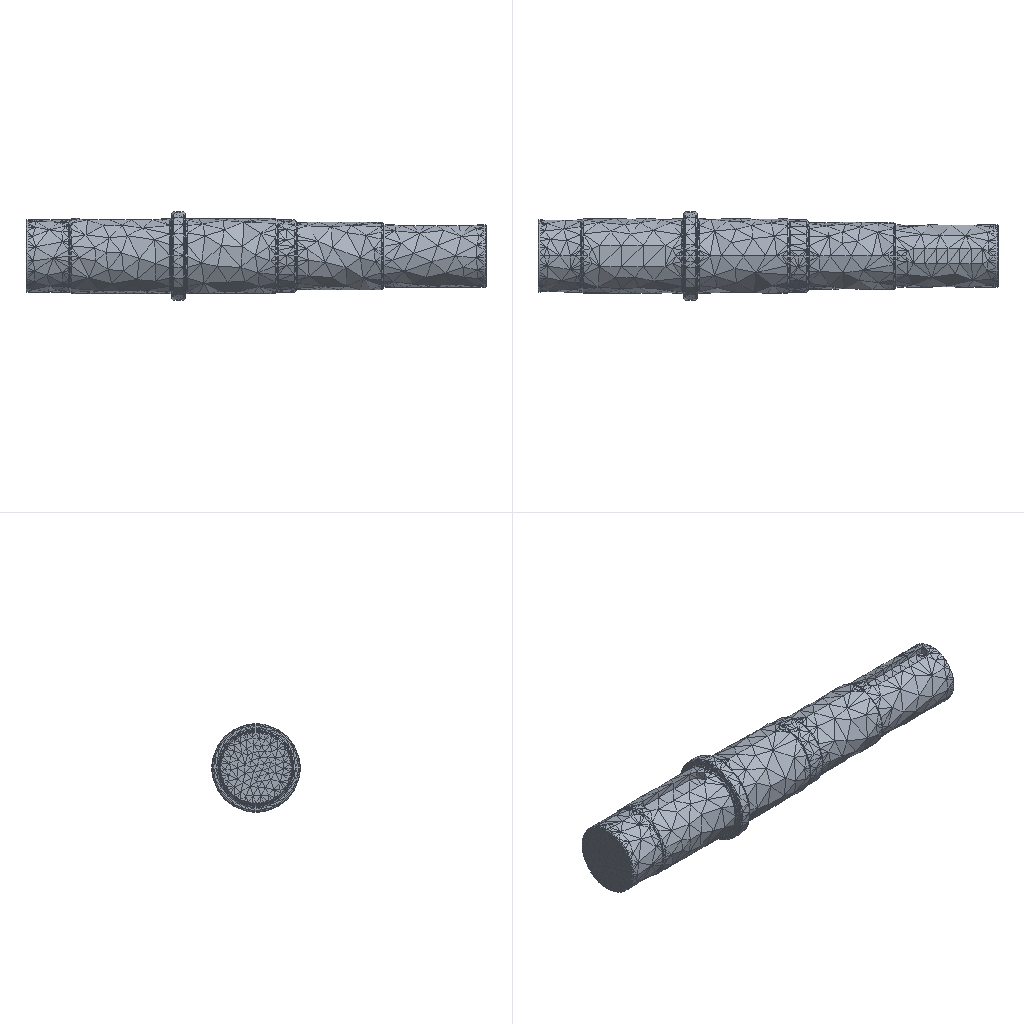Simulation study | ansys workbench
Ansys APDL input file, long lists of numbers shortened:
/batch
/config,noeldb,1     ! force off writing results to database
*get,_wallstrt,active,,time,wall
! ANSYS input file written by Workbench version 2022 R1
! File used for geometry attach: F:\ansys（分析文件汇总)\轴有限元分析222\三轴.STEP
/title,1--____ (B5)
! ****** Begin Custom Load Command Snippet ******
/COM, ACT Extensions:
/COM,     LSDYNA, 2021.1
/COM,
! ****** End   Custom Load Command Snippet ******
*DIM,_wb_ProjectScratch_dir,string,248
_wb_ProjectScratch_dir(1) = 'F:\ansys（分析文件汇总)\轴有限元分析222\_ProjectScratch\Scr97E6\'
*DIM,_wb_SolverFiles_dir,string,248
_wb_SolverFiles_dir(1) = 'F:\ansys（分析文件汇总)\轴有限元分析222\1_files\dp0\SYS\MECH\'
*DIM,_wb_userfiles_dir,string,248
_wb_userfiles_dir(1) = 'F:\ansys（分析文件汇总)\轴有限元分析222\1_files\user_files\'
/com,--- Data in consistent NMM units. See Solving Units in the help system for more information.
/units,MPA
/nopr
/wb,file,start              !  signify a WB generated input file
/prep7
! Turn off shape checking because checks already performed inside WB mesher.
! See help system for more information.
SHPP,OFF,,NOWARN
/nolist
etcon,set             ! allow ANSYS to choose best KEYOP's for 180x elements, resets any applicable keyopt to MAPDL defaults
/com,*********** Nodes for the whole assembly ***********
nblock,3,,12992
(1i9,3e20.9e3)
        1     1.495000000E+02     6.024925164E-25    -3.900000000E+01
! (11810 more lines like these left out)
-1
/com,*********** Nodes for all Remote Points ***********
nblock,3
(1i9,3e20.9e3)
    11812     2.186806849E+02    -4.529709940E-14    -2.585144555E-16
-1
/wb,elem,start            !  set before creation of elements
/com,*********** Elements for Body 1 "__-FreeParts|0:35179" ***********
et,1,187
eblock,19,solid,,6720
(19i9)
        1        1        1        1        0        0        0        0       10        0        1      349     1869      691     1621     4224     6255     4217     4221
! (13439 more lines like these left out)
-1
/wb,elem,end               !  done creating elements
/com,*********** Send User Defined Coordinate System(s) ***********
csys,0
toffst,273.15,  ! Temperature offset from absolute zero
/com,*********** Set Reference Temperature ***********
tref,22.
/wb,mat,start              !  starting to send materials
/com,*********** Send Materials ***********
Temperature = 'TEMP' ! Temperature
MP,DENS,1,7.85e-09,	! tonne mm^-3
MP,ALPX,1,1.2e-05,	! C^-1
MP,C,1,434000000,	! mm^2 s^-2 C^-1
MP,KXX,1,60.5,	! tonne mm s^-3 C^-1
MP,RSVX,1,0.00017,	! ohm mm
MP,EX,1,200000,	! tonne s^-2 mm^-1
MP,NUXY,1,0.3,
MP,MURX,1,10000,
/wb,mat,end                !  done sending materials
!************************* Model Summary ********************
!__-FreeParts|0:35179,	结构钢,	matid,	1
!************************* End Model Summary ********************
! get the diagonal of the bounding box. Needed later for other things
*get,_xmin,node,,mnloc,x
*get,_ymin,node,,mnloc,y
*get,_zmin,node,,mnloc,z
*get,_xmax,node,,mxloc,x
*get,_ymax,node,,mxloc,y
*get,_zmax,node,,mxloc,z
_ASMDIAG=(_xmax-_xmin)*(_xmax-_xmin)+(_ymax-_ymin)*(_ymax-_ymin)+(_zmax-_zmin)*(_zmax-_zmin)
_ASMDIAG=SQRT(_ASMDIAG)
/wb,contact,start          !  starting to send contact
/wb,contact,end            !  done creating contacts
/golist
/wb,load,start             !  starting to send loads
/com,*********** Fixed Supports ***********
CMBLOCK,_FIXEDSU,NODE,      971
(8i10)
         1         4         5         6         7         8        96        99
! (121 more lines like these left out)
cmsel,s,_FIXEDSU
d,all,all
nsel,all
/com,*********** Create Remote Point "内部远程点" ***********
! -------- Remote Point Used by "力矩" --------
*set,tid,3
*set,cid,2
et,cid,174
et,tid,170
keyo,tid,2,1               ! Don't fix the pilot node
keyo,tid,4,111111
keyo,cid,12,5              ! Bonded Contact
keyo,cid,4,1               ! Deformable RBE3 style load
keyo,cid,2,2               ! MPC style contact
eblock,10,,,455
(15i9)
     9378        2        2        2        0      140      463      800      800     2949     5026      800     2950
! (454 more lines like these left out)
-1
*set,_npilot,11812
_npilot32=_npilot
type,tid
mat ,cid
real,cid
tshape,pilo
en,9833,_npilot
tshape
/com,*********** Construct Moment Using Remote Attachment ***********
/gst,on,on
fini
*get,_numnode,node,0,count
*get,_numelem,elem,0,count
*get, _MAXELEMNUM, elem, 0, NUM, MAX
*get, _MAXNODENUM, node, 0, NUM, MAX
*get, _MAXELEMTYPE, etyp, 0, NUM, MAX
*get, _MAXREALCONST, real, 0, NUM, MAX
/go
/wb,load,end               !  done creating loads
/com,--- Number of total nodes = %_numnode%
/com,--- Number of contact elements = 455
/com,--- Number of spring elements = 0
/com,--- Number of bearing elements = 0
/com,--- Number of solid elements = 6720
/com,--- Number of condensed parts = 0
/com,--- Number of total elements = %_numelem%
*get,_wallbsol,active,,time,wall
/com,****************************************************************************
/com,*************************    SOLUTION       ********************************
/com,****************************************************************************
/solu
antype,0                   ! static analysis
_thickRatio=  1     ! Ratio of thick parts in the model
eqsl,pcg,1e-8,,,,,,1
cntr,print,1               ! print out contact info and also make no initial contact an error
dmpoption,emat,no             ! Don't combine emat file for DANSYS
dmpoption,esav,no             ! Don't combine esav file for DANSYS
nldiag,cont,iter           ! print out contact info each equilibrium iteration
rescontrol,,none                 ! Do not keep any restart files
/com,****************************************************
/com,******************* SOLVE FOR LS 1 OF 1 ****************
nsel,s,node,,11812
f,all,mx,900000.
f,all,my,0.
f,all,mz,0.
nsel,all
/nopr
/gopr
nsub,1,1,1
time,1.
outres,erase
outres,all,none
outres,nsol,all,
outres,rsol,all
outres,eangl,all
outres,etmp,all
outres,veng,all
outres,strs,all,
outres,epel,all,
outres,eppl,all,
outres,cont,all,
! *********** WB SOLVE COMMAND ***********
! check interactive state
*get,ANSINTER_,active,,int
*if,ANSINTER_,ne,0,then
/eof
*endif
solve
/com *************** Write FE CONNECTORS *********
CEWRITE,file,ce,,INTE
/com,****************************************************
/com,*************** FINISHED SOLVE FOR LS 1 *************
*get,_wallasol,active,,time,wall
/nopr
*get,_numnode,node,0,count
*get,_numelem,elem,0,count
*get, _MAXELEMNUM, elem, 0, NUM, MAX
*get, _MAXNODENUM, node, 0, NUM, MAX,,,INTERNAL
*get, _MAXELEMTYPE, etyp, 0, NUM, MAX
*get, _MAXREALCONST, real, 0, NUM, MAX
/gopr
*get,_PCGITER,active,,solu,cgiter
/post1
xmlo,ENCODING,ISO-8859-1
xmlo,parm
/xml,parm,xml
fini
/gopr
*get,_walldone,active,,time,wall
_preptime=(_wallbsol-_wallstrt)*3600
_solvtime=(_wallasol-_wallbsol)*3600
_posttime=(_walldone-_wallasol)*3600
_totaltim=(_walldone-_wallstrt)*3600
*get,_dlbratio,active,0,solu,dlbr
*get,_combtime,active,0,solu,comb
*get,_ssmode,active,0,solu,ssmm
*get,_ndofs,active,0,solu,ndof
*get,_sol_end_time,active,0,set,time
*if,_sol_end_time,eq,1.,then
/fclean				!clean distributed files
*endif
/com,--- Total number of nodes = %_numnode%
/com,--- Total number of elements = %_numelem%
/com,--- Element load balance ratio = %_dlbratio%
/com,--- Time to combine distributed files = %_combtime%
/com,--- Sparse memory mode = %_ssmode%
/com,--- Number of DOF = %_ndofs%
/wb,file,end               ! done with WB generated input